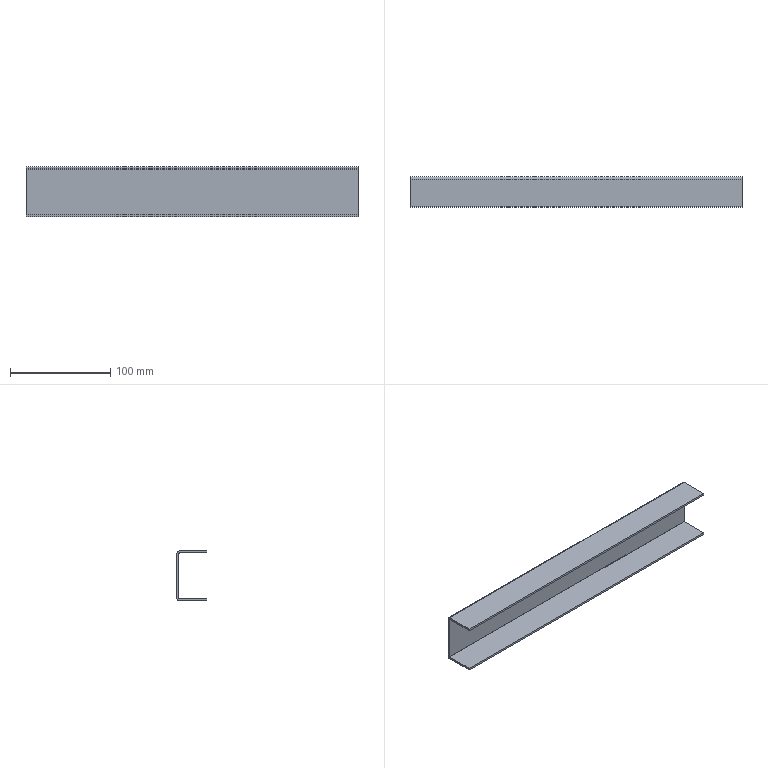Part | SolidWorks | 1 solid | 22 faces | box 332 x 30 x 50 mm | volume 69757 mm3 | plane 18 | cylinder 4 | commonest cylinder face diameters 0.2 x2 4.2 x2
STEP:
#1=CARTESIAN_POINT('',(166.,0.,-2.1));
#2=VERTEX_POINT('',#1);
#3=CARTESIAN_POINT('',(166.,-2.,-2.1));
#4=VERTEX_POINT('',#3);
#5=CARTESIAN_POINT('',(166.,0.,-2.1));
#6=DIRECTION('',(0.,-1.,0.));
#7=VECTOR('',#6,1000.);
#8=LINE('',#5,#7);
#9=EDGE_CURVE('',#2,#4,#8,.T.);
#10=ORIENTED_EDGE('',*,*,#9,.F.);
#11=CARTESIAN_POINT('',(166.,-2.1,0.));
#12=VERTEX_POINT('',#11);
#13=CARTESIAN_POINT('',(166.,-2.1,-2.1));
#14=DIRECTION('',(1.,0.,0.));
#15=DIRECTION('',(0.,0.,-1.));
#16=AXIS2_PLACEMENT_3D('',#13,#14,#15);
#17=CIRCLE('',#16,2.1);
#18=EDGE_CURVE('',#2,#12,#17,.T.);
#19=ORIENTED_EDGE('',*,*,#18,.T.);
#20=CARTESIAN_POINT('',(166.,-2.1,-2.));
#21=VERTEX_POINT('',#20);
#22=CARTESIAN_POINT('',(166.,-2.1,-2.));
#23=DIRECTION('',(0.,0.,1.));
#24=VECTOR('',#23,1000.);
#25=LINE('',#22,#24);
#26=EDGE_CURVE('',#21,#12,#25,.T.);
#27=ORIENTED_EDGE('',*,*,#26,.F.);
#28=CARTESIAN_POINT('',(166.,-2.1,-2.1));
#29=DIRECTION('',(1.,0.,0.));
#30=DIRECTION('',(0.,0.,-1.));
#31=AXIS2_PLACEMENT_3D('',#28,#29,#30);
#32=CIRCLE('',#31,0.1);
#33=EDGE_CURVE('',#4,#21,#32,.T.);
#34=ORIENTED_EDGE('',*,*,#33,.F.);
#35=EDGE_LOOP('',(#10,#19,#27,#34));
#36=FACE_OUTER_BOUND('',#35,.T.);
#37=CARTESIAN_POINT('',(166.,0.,-2.1));
#38=DIRECTION('',(1.,0.,0.));
#39=DIRECTION('',(0.,0.,-1.));
#40=AXIS2_PLACEMENT_3D('',#37,#38,#39);
#41=PLANE('',#40);
#42=ADVANCED_FACE('',(#36),#41,.T.);
#43=CARTESIAN_POINT('',(166.,0.,-47.9));
#44=VERTEX_POINT('',#43);
#45=CARTESIAN_POINT('',(166.,0.,0.));
#46=DIRECTION('',(0.,0.,1.));
#47=VECTOR('',#46,1000.);
#48=LINE('',#45,#47);
#49=EDGE_CURVE('',#44,#2,#48,.T.);
#50=ORIENTED_EDGE('',*,*,#49,.T.);
#51=ORIENTED_EDGE('',*,*,#9,.T.);
#52=CARTESIAN_POINT('',(166.,-2.,-47.9));
#53=VERTEX_POINT('',#52);
#54=CARTESIAN_POINT('',(166.,-2.,0.));
#55=DIRECTION('',(0.,0.,1.));
#56=VECTOR('',#55,1000.);
#57=LINE('',#54,#56);
#58=EDGE_CURVE('',#53,#4,#57,.T.);
#59=ORIENTED_EDGE('',*,*,#58,.F.);
#60=CARTESIAN_POINT('',(166.,-2.,-47.9));
#61=DIRECTION('',(0.,1.,0.));
#62=VECTOR('',#61,1000.);
#63=LINE('',#60,#62);
#64=EDGE_CURVE('',#53,#44,#63,.T.);
#65=ORIENTED_EDGE('',*,*,#64,.T.);
#66=EDGE_LOOP('',(#50,#51,#59,#65));
#67=FACE_OUTER_BOUND('',#66,.T.);
#68=CARTESIAN_POINT('',(166.,-2.1,-2.));
#69=DIRECTION('',(1.,0.,0.));
#70=DIRECTION('',(0.,0.,-1.));
#71=AXIS2_PLACEMENT_3D('',#68,#69,#70);
#72=PLANE('',#71);
#73=ADVANCED_FACE('',(#67),#72,.T.);
#74=CARTESIAN_POINT('',(-166.,-2.1,0.));
#75=VERTEX_POINT('',#74);
#76=CARTESIAN_POINT('',(-166.,-2.1,-2.));
#77=VERTEX_POINT('',#76);
#78=CARTESIAN_POINT('',(-166.,-2.1,0.));
#79=DIRECTION('',(0.,0.,-1.));
#80=VECTOR('',#79,1000.);
#81=LINE('',#78,#80);
#82=EDGE_CURVE('',#75,#77,#81,.T.);
#83=ORIENTED_EDGE('',*,*,#82,.F.);
#84=CARTESIAN_POINT('',(-166.,0.,-2.1));
#85=VERTEX_POINT('',#84);
#86=CARTESIAN_POINT('',(-166.,-2.1,-2.1));
#87=DIRECTION('',(1.,0.,0.));
#88=DIRECTION('',(0.,0.,-1.));
#89=AXIS2_PLACEMENT_3D('',#86,#87,#88);
#90=CIRCLE('',#89,2.1);
#91=EDGE_CURVE('',#85,#75,#90,.T.);
#92=ORIENTED_EDGE('',*,*,#91,.F.);
#93=CARTESIAN_POINT('',(-166.,-2.,-2.1));
#94=VERTEX_POINT('',#93);
#95=CARTESIAN_POINT('',(-166.,-2.,-2.1));
#96=DIRECTION('',(0.,1.,0.));
#97=VECTOR('',#96,1000.);
#98=LINE('',#95,#97);
#99=EDGE_CURVE('',#94,#85,#98,.T.);
#100=ORIENTED_EDGE('',*,*,#99,.F.);
#101=CARTESIAN_POINT('',(-166.,-2.1,-2.1));
#102=DIRECTION('',(1.,0.,0.));
#103=DIRECTION('',(0.,0.,-1.));
#104=AXIS2_PLACEMENT_3D('',#101,#102,#103);
#105=CIRCLE('',#104,0.1);
#106=EDGE_CURVE('',#94,#77,#105,.T.);
#107=ORIENTED_EDGE('',*,*,#106,.T.);
#108=EDGE_LOOP('',(#83,#92,#100,#107));
#109=FACE_OUTER_BOUND('',#108,.T.);
#110=CARTESIAN_POINT('',(-166.,-2.1,0.));
#111=DIRECTION('',(-1.,0.,0.));
#112=DIRECTION('',(0.,0.,1.));
#113=AXIS2_PLACEMENT_3D('',#110,#111,#112);
#114=PLANE('',#113);
#115=ADVANCED_FACE('',(#109),#114,.T.);
#116=CARTESIAN_POINT('',(-166.,-30.,0.));
#117=VERTEX_POINT('',#116);
#118=CARTESIAN_POINT('',(-166.,0.,0.));
#119=DIRECTION('',(0.,-1.,0.));
#120=VECTOR('',#119,1000.);
#121=LINE('',#118,#120);
#122=EDGE_CURVE('',#75,#117,#121,.T.);
#123=ORIENTED_EDGE('',*,*,#122,.F.);
#124=ORIENTED_EDGE('',*,*,#82,.T.);
#125=CARTESIAN_POINT('',(-166.,-30.,-2.));
#126=VERTEX_POINT('',#125);
#127=CARTESIAN_POINT('',(-166.,0.,-2.));
#128=DIRECTION('',(0.,-1.,0.));
#129=VECTOR('',#128,1000.);
#130=LINE('',#127,#129);
#131=EDGE_CURVE('',#77,#126,#130,.T.);
#132=ORIENTED_EDGE('',*,*,#131,.T.);
#133=CARTESIAN_POINT('',(-166.,-30.,-2.));
#134=DIRECTION('',(0.,0.,1.));
#135=VECTOR('',#134,1000.);
#136=LINE('',#133,#135);
#137=EDGE_CURVE('',#126,#117,#136,.T.);
#138=ORIENTED_EDGE('',*,*,#137,.T.);
#139=EDGE_LOOP('',(#123,#124,#132,#138));
#140=FACE_OUTER_BOUND('',#139,.T.);
#141=CARTESIAN_POINT('',(-166.,-2.,-2.1));
#142=DIRECTION('',(-1.,0.,0.));
#143=DIRECTION('',(0.,0.,1.));
#144=AXIS2_PLACEMENT_3D('',#141,#142,#143);
#145=PLANE('',#144);
#146=ADVANCED_FACE('',(#140),#145,.T.);
#147=CARTESIAN_POINT('',(166.,-2.1,-50.));
#148=VERTEX_POINT('',#147);
#149=CARTESIAN_POINT('',(166.,-2.1,-48.));
#150=VERTEX_POINT('',#149);
#151=CARTESIAN_POINT('',(166.,-2.1,-50.));
#152=DIRECTION('',(0.,0.,1.));
#153=VECTOR('',#152,1000.);
#154=LINE('',#151,#153);
#155=EDGE_CURVE('',#148,#150,#154,.T.);
#156=ORIENTED_EDGE('',*,*,#155,.F.);
#157=CARTESIAN_POINT('',(166.,-2.1,-47.9));
#158=DIRECTION('',(1.,0.,0.));
#159=DIRECTION('',(0.,0.,-1.));
#160=AXIS2_PLACEMENT_3D('',#157,#158,#159);
#161=CIRCLE('',#160,2.1);
#162=EDGE_CURVE('',#148,#44,#161,.T.);
#163=ORIENTED_EDGE('',*,*,#162,.T.);
#164=ORIENTED_EDGE('',*,*,#64,.F.);
#165=CARTESIAN_POINT('',(166.,-2.1,-47.9));
#166=DIRECTION('',(1.,0.,0.));
#167=DIRECTION('',(0.,0.,-1.));
#168=AXIS2_PLACEMENT_3D('',#165,#166,#167);
#169=CIRCLE('',#168,0.1);
#170=EDGE_CURVE('',#150,#53,#169,.T.);
#171=ORIENTED_EDGE('',*,*,#170,.F.);
#172=EDGE_LOOP('',(#156,#163,#164,#171));
#173=FACE_OUTER_BOUND('',#172,.T.);
#174=CARTESIAN_POINT('',(166.,-2.1,-50.));
#175=DIRECTION('',(1.,0.,0.));
#176=DIRECTION('',(0.,0.,-1.));
#177=AXIS2_PLACEMENT_3D('',#174,#175,#176);
#178=PLANE('',#177);
#179=ADVANCED_FACE('',(#173),#178,.T.);
#180=CARTESIAN_POINT('',(166.,-30.,-50.));
#181=VERTEX_POINT('',#180);
#182=CARTESIAN_POINT('',(166.,0.,-50.));
#183=DIRECTION('',(0.,1.,0.));
#184=VECTOR('',#183,1000.);
#185=LINE('',#182,#184);
#186=EDGE_CURVE('',#181,#148,#185,.T.);
#187=ORIENTED_EDGE('',*,*,#186,.T.);
#188=ORIENTED_EDGE('',*,*,#155,.T.);
#189=CARTESIAN_POINT('',(166.,-30.,-48.));
#190=VERTEX_POINT('',#189);
#191=CARTESIAN_POINT('',(166.,0.,-48.));
#192=DIRECTION('',(0.,1.,0.));
#193=VECTOR('',#192,1000.);
#194=LINE('',#191,#193);
#195=EDGE_CURVE('',#190,#150,#194,.T.);
#196=ORIENTED_EDGE('',*,*,#195,.F.);
#197=CARTESIAN_POINT('',(166.,-30.,-50.));
#198=DIRECTION('',(0.,0.,1.));
#199=VECTOR('',#198,1000.);
#200=LINE('',#197,#199);
#201=EDGE_CURVE('',#181,#190,#200,.T.);
#202=ORIENTED_EDGE('',*,*,#201,.F.);
#203=EDGE_LOOP('',(#187,#188,#196,#202));
#204=FACE_OUTER_BOUND('',#203,.T.);
#205=CARTESIAN_POINT('',(166.,-2.,-47.9));
#206=DIRECTION('',(1.,0.,0.));
#207=DIRECTION('',(0.,0.,-1.));
#208=AXIS2_PLACEMENT_3D('',#205,#206,#207);
#209=PLANE('',#208);
#210=ADVANCED_FACE('',(#204),#209,.T.);
#211=CARTESIAN_POINT('',(-166.,0.,-47.9));
#212=VERTEX_POINT('',#211);
#213=CARTESIAN_POINT('',(-166.,-2.,-47.9));
#214=VERTEX_POINT('',#213);
#215=CARTESIAN_POINT('',(-166.,0.,-47.9));
#216=DIRECTION('',(0.,-1.,0.));
#217=VECTOR('',#216,1000.);
#218=LINE('',#215,#217);
#219=EDGE_CURVE('',#212,#214,#218,.T.);
#220=ORIENTED_EDGE('',*,*,#219,.F.);
#221=CARTESIAN_POINT('',(-166.,-2.1,-50.));
#222=VERTEX_POINT('',#221);
#223=CARTESIAN_POINT('',(-166.,-2.1,-47.9));
#224=DIRECTION('',(1.,0.,0.));
#225=DIRECTION('',(0.,0.,-1.));
#226=AXIS2_PLACEMENT_3D('',#223,#224,#225);
#227=CIRCLE('',#226,2.1);
#228=EDGE_CURVE('',#222,#212,#227,.T.);
#229=ORIENTED_EDGE('',*,*,#228,.F.);
#230=CARTESIAN_POINT('',(-166.,-2.1,-48.));
#231=VERTEX_POINT('',#230);
#232=CARTESIAN_POINT('',(-166.,-2.1,-48.));
#233=DIRECTION('',(0.,0.,-1.));
#234=VECTOR('',#233,1000.);
#235=LINE('',#232,#234);
#236=EDGE_CURVE('',#231,#222,#235,.T.);
#237=ORIENTED_EDGE('',*,*,#236,.F.);
#238=CARTESIAN_POINT('',(-166.,-2.1,-47.9));
#239=DIRECTION('',(1.,0.,0.));
#240=DIRECTION('',(0.,0.,-1.));
#241=AXIS2_PLACEMENT_3D('',#238,#239,#240);
#242=CIRCLE('',#241,0.1);
#243=EDGE_CURVE('',#231,#214,#242,.T.);
#244=ORIENTED_EDGE('',*,*,#243,.T.);
#245=EDGE_LOOP('',(#220,#229,#237,#244));
#246=FACE_OUTER_BOUND('',#245,.T.);
#247=CARTESIAN_POINT('',(-166.,0.,-47.9));
#248=DIRECTION('',(-1.,0.,0.));
#249=DIRECTION('',(0.,0.,1.));
#250=AXIS2_PLACEMENT_3D('',#247,#248,#249);
#251=PLANE('',#250);
#252=ADVANCED_FACE('',(#246),#251,.T.);
#253=CARTESIAN_POINT('',(-166.,0.,0.));
#254=DIRECTION('',(0.,0.,1.));
#255=VECTOR('',#254,1000.);
#256=LINE('',#253,#255);
#257=EDGE_CURVE('',#212,#85,#256,.T.);
#258=ORIENTED_EDGE('',*,*,#257,.F.);
#259=ORIENTED_EDGE('',*,*,#219,.T.);
#260=CARTESIAN_POINT('',(-166.,-2.,0.));
#261=DIRECTION('',(0.,0.,1.));
#262=VECTOR('',#261,1000.);
#263=LINE('',#260,#262);
#264=EDGE_CURVE('',#214,#94,#263,.T.);
#265=ORIENTED_EDGE('',*,*,#264,.T.);
#266=ORIENTED_EDGE('',*,*,#99,.T.);
#267=EDGE_LOOP('',(#258,#259,#265,#266));
#268=FACE_OUTER_BOUND('',#267,.T.);
#269=CARTESIAN_POINT('',(-166.,-2.1,-48.));
#270=DIRECTION('',(-1.,0.,0.));
#271=DIRECTION('',(0.,0.,1.));
#272=AXIS2_PLACEMENT_3D('',#269,#270,#271);
#273=PLANE('',#272);
#274=ADVANCED_FACE('',(#268),#273,.T.);
#275=ORIENTED_EDGE('',*,*,#122,.T.);
#276=CARTESIAN_POINT('',(166.,-30.,0.));
#277=VERTEX_POINT('',#276);
#278=CARTESIAN_POINT('',(166.,-30.,0.));
#279=DIRECTION('',(-1.,0.,0.));
#280=VECTOR('',#279,1000.);
#281=LINE('',#278,#280);
#282=EDGE_CURVE('',#277,#117,#281,.T.);
#283=ORIENTED_EDGE('',*,*,#282,.F.);
#284=CARTESIAN_POINT('',(166.,0.,0.));
#285=DIRECTION('',(0.,-1.,0.));
#286=VECTOR('',#285,1000.);
#287=LINE('',#284,#286);
#288=EDGE_CURVE('',#12,#277,#287,.T.);
#289=ORIENTED_EDGE('',*,*,#288,.F.);
#290=CARTESIAN_POINT('',(166.,-2.1,0.));
#291=DIRECTION('',(-1.,0.,0.));
#292=VECTOR('',#291,1000.);
#293=LINE('',#290,#292);
#294=EDGE_CURVE('',#12,#75,#293,.T.);
#295=ORIENTED_EDGE('',*,*,#294,.T.);
#296=EDGE_LOOP('',(#275,#283,#289,#295));
#297=FACE_OUTER_BOUND('',#296,.T.);
#298=CARTESIAN_POINT('',(166.,0.,0.));
#299=DIRECTION('',(0.,0.,-1.));
#300=DIRECTION('',(0.,1.,0.));
#301=AXIS2_PLACEMENT_3D('',#298,#299,#300);
#302=PLANE('',#301);
#303=ADVANCED_FACE('',(#297),#302,.F.);
#304=ORIENTED_EDGE('',*,*,#137,.F.);
#305=CARTESIAN_POINT('',(166.,-30.,-2.));
#306=VERTEX_POINT('',#305);
#307=CARTESIAN_POINT('',(166.,-30.,-2.));
#308=DIRECTION('',(-1.,0.,0.));
#309=VECTOR('',#308,1000.);
#310=LINE('',#307,#309);
#311=EDGE_CURVE('',#306,#126,#310,.T.);
#312=ORIENTED_EDGE('',*,*,#311,.F.);
#313=CARTESIAN_POINT('',(166.,-30.,-2.));
#314=DIRECTION('',(0.,0.,1.));
#315=VECTOR('',#314,1000.);
#316=LINE('',#313,#315);
#317=EDGE_CURVE('',#306,#277,#316,.T.);
#318=ORIENTED_EDGE('',*,*,#317,.T.);
#319=ORIENTED_EDGE('',*,*,#282,.T.);
#320=EDGE_LOOP('',(#304,#312,#318,#319));
#321=FACE_OUTER_BOUND('',#320,.T.);
#322=CARTESIAN_POINT('',(166.,-30.,-2.));
#323=DIRECTION('',(0.,-1.,0.));
#324=DIRECTION('',(0.,0.,-1.));
#325=AXIS2_PLACEMENT_3D('',#322,#323,#324);
#326=PLANE('',#325);
#327=ADVANCED_FACE('',(#321),#326,.T.);
#328=ORIENTED_EDGE('',*,*,#131,.F.);
#329=CARTESIAN_POINT('',(166.,-2.1,-2.));
#330=DIRECTION('',(-1.,0.,0.));
#331=VECTOR('',#330,1000.);
#332=LINE('',#329,#331);
#333=EDGE_CURVE('',#21,#77,#332,.T.);
#334=ORIENTED_EDGE('',*,*,#333,.F.);
#335=CARTESIAN_POINT('',(166.,0.,-2.));
#336=DIRECTION('',(0.,-1.,0.));
#337=VECTOR('',#336,1000.);
#338=LINE('',#335,#337);
#339=EDGE_CURVE('',#21,#306,#338,.T.);
#340=ORIENTED_EDGE('',*,*,#339,.T.);
#341=ORIENTED_EDGE('',*,*,#311,.T.);
#342=EDGE_LOOP('',(#328,#334,#340,#341));
#343=FACE_OUTER_BOUND('',#342,.T.);
#344=CARTESIAN_POINT('',(166.,0.,-2.));
#345=DIRECTION('',(0.,0.,-1.));
#346=DIRECTION('',(0.,1.,0.));
#347=AXIS2_PLACEMENT_3D('',#344,#345,#346);
#348=PLANE('',#347);
#349=ADVANCED_FACE('',(#343),#348,.T.);
#350=ORIENTED_EDGE('',*,*,#106,.F.);
#351=CARTESIAN_POINT('',(166.,-2.,-2.1));
#352=DIRECTION('',(-1.,0.,0.));
#353=VECTOR('',#352,1000.);
#354=LINE('',#351,#353);
#355=EDGE_CURVE('',#4,#94,#354,.T.);
#356=ORIENTED_EDGE('',*,*,#355,.F.);
#357=ORIENTED_EDGE('',*,*,#33,.T.);
#358=ORIENTED_EDGE('',*,*,#333,.T.);
#359=EDGE_LOOP('',(#350,#356,#357,#358));
#360=FACE_OUTER_BOUND('',#359,.T.);
#361=CARTESIAN_POINT('',(166.,-2.1,-2.1));
#362=DIRECTION('',(-1.,0.,0.));
#363=DIRECTION('',(0.,0.,1.));
#364=AXIS2_PLACEMENT_3D('',#361,#362,#363);
#365=CYLINDRICAL_SURFACE('',#364,0.1);
#366=ADVANCED_FACE('',(#360),#365,.F.);
#367=ORIENTED_EDGE('',*,*,#264,.F.);
#368=CARTESIAN_POINT('',(166.,-2.,-47.9));
#369=DIRECTION('',(-1.,0.,0.));
#370=VECTOR('',#369,1000.);
#371=LINE('',#368,#370);
#372=EDGE_CURVE('',#53,#214,#371,.T.);
#373=ORIENTED_EDGE('',*,*,#372,.F.);
#374=ORIENTED_EDGE('',*,*,#58,.T.);
#375=ORIENTED_EDGE('',*,*,#355,.T.);
#376=EDGE_LOOP('',(#367,#373,#374,#375));
#377=FACE_OUTER_BOUND('',#376,.T.);
#378=CARTESIAN_POINT('',(166.,-2.,0.));
#379=DIRECTION('',(0.,-1.,0.));
#380=DIRECTION('',(0.,0.,-1.));
#381=AXIS2_PLACEMENT_3D('',#378,#379,#380);
#382=PLANE('',#381);
#383=ADVANCED_FACE('',(#377),#382,.T.);
#384=ORIENTED_EDGE('',*,*,#243,.F.);
#385=CARTESIAN_POINT('',(166.,-2.1,-48.));
#386=DIRECTION('',(-1.,0.,0.));
#387=VECTOR('',#386,1000.);
#388=LINE('',#385,#387);
#389=EDGE_CURVE('',#150,#231,#388,.T.);
#390=ORIENTED_EDGE('',*,*,#389,.F.);
#391=ORIENTED_EDGE('',*,*,#170,.T.);
#392=ORIENTED_EDGE('',*,*,#372,.T.);
#393=EDGE_LOOP('',(#384,#390,#391,#392));
#394=FACE_OUTER_BOUND('',#393,.T.);
#395=CARTESIAN_POINT('',(166.,-2.1,-47.9));
#396=DIRECTION('',(-1.,0.,0.));
#397=DIRECTION('',(0.,0.,1.));
#398=AXIS2_PLACEMENT_3D('',#395,#396,#397);
#399=CYLINDRICAL_SURFACE('',#398,0.1);
#400=ADVANCED_FACE('',(#394),#399,.F.);
#401=CARTESIAN_POINT('',(-166.,-30.,-48.));
#402=VERTEX_POINT('',#401);
#403=CARTESIAN_POINT('',(-166.,0.,-48.));
#404=DIRECTION('',(0.,1.,0.));
#405=VECTOR('',#404,1000.);
#406=LINE('',#403,#405);
#407=EDGE_CURVE('',#402,#231,#406,.T.);
#408=ORIENTED_EDGE('',*,*,#407,.F.);
#409=CARTESIAN_POINT('',(166.,-30.,-48.));
#410=DIRECTION('',(-1.,0.,0.));
#411=VECTOR('',#410,1000.);
#412=LINE('',#409,#411);
#413=EDGE_CURVE('',#190,#402,#412,.T.);
#414=ORIENTED_EDGE('',*,*,#413,.F.);
#415=ORIENTED_EDGE('',*,*,#195,.T.);
#416=ORIENTED_EDGE('',*,*,#389,.T.);
#417=EDGE_LOOP('',(#408,#414,#415,#416));
#418=FACE_OUTER_BOUND('',#417,.T.);
#419=CARTESIAN_POINT('',(166.,0.,-48.));
#420=DIRECTION('',(0.,0.,1.));
#421=DIRECTION('',(0.,-1.,0.));
#422=AXIS2_PLACEMENT_3D('',#419,#420,#421);
#423=PLANE('',#422);
#424=ADVANCED_FACE('',(#418),#423,.T.);
#425=CARTESIAN_POINT('',(-166.,-30.,-50.));
#426=VERTEX_POINT('',#425);
#427=CARTESIAN_POINT('',(-166.,-30.,-50.));
#428=DIRECTION('',(0.,0.,1.));
#429=VECTOR('',#428,1000.);
#430=LINE('',#427,#429);
#431=EDGE_CURVE('',#426,#402,#430,.T.);
#432=ORIENTED_EDGE('',*,*,#431,.F.);
#433=CARTESIAN_POINT('',(166.,-30.,-50.));
#434=DIRECTION('',(-1.,0.,0.));
#435=VECTOR('',#434,1000.);
#436=LINE('',#433,#435);
#437=EDGE_CURVE('',#181,#426,#436,.T.);
#438=ORIENTED_EDGE('',*,*,#437,.F.);
#439=ORIENTED_EDGE('',*,*,#201,.T.);
#440=ORIENTED_EDGE('',*,*,#413,.T.);
#441=EDGE_LOOP('',(#432,#438,#439,#440));
#442=FACE_OUTER_BOUND('',#441,.T.);
#443=CARTESIAN_POINT('',(166.,-30.,-50.));
#444=DIRECTION('',(0.,-1.,0.));
#445=DIRECTION('',(0.,0.,-1.));
#446=AXIS2_PLACEMENT_3D('',#443,#444,#445);
#447=PLANE('',#446);
#448=ADVANCED_FACE('',(#442),#447,.T.);
#449=CARTESIAN_POINT('',(-166.,0.,-50.));
#450=DIRECTION('',(0.,1.,0.));
#451=VECTOR('',#450,1000.);
#452=LINE('',#449,#451);
#453=EDGE_CURVE('',#426,#222,#452,.T.);
#454=ORIENTED_EDGE('',*,*,#453,.T.);
#455=CARTESIAN_POINT('',(166.,-2.1,-50.));
#456=DIRECTION('',(-1.,0.,0.));
#457=VECTOR('',#456,1000.);
#458=LINE('',#455,#457);
#459=EDGE_CURVE('',#148,#222,#458,.T.);
#460=ORIENTED_EDGE('',*,*,#459,.F.);
#461=ORIENTED_EDGE('',*,*,#186,.F.);
#462=ORIENTED_EDGE('',*,*,#437,.T.);
#463=EDGE_LOOP('',(#454,#460,#461,#462));
#464=FACE_OUTER_BOUND('',#463,.T.);
#465=CARTESIAN_POINT('',(166.,0.,-50.));
#466=DIRECTION('',(0.,0.,1.));
#467=DIRECTION('',(0.,-1.,0.));
#468=AXIS2_PLACEMENT_3D('',#465,#466,#467);
#469=PLANE('',#468);
#470=ADVANCED_FACE('',(#464),#469,.F.);
#471=ORIENTED_EDGE('',*,*,#228,.T.);
#472=CARTESIAN_POINT('',(166.,0.,-47.9));
#473=DIRECTION('',(-1.,0.,0.));
#474=VECTOR('',#473,1000.);
#475=LINE('',#472,#474);
#476=EDGE_CURVE('',#44,#212,#475,.T.);
#477=ORIENTED_EDGE('',*,*,#476,.F.);
#478=ORIENTED_EDGE('',*,*,#162,.F.);
#479=ORIENTED_EDGE('',*,*,#459,.T.);
#480=EDGE_LOOP('',(#471,#477,#478,#479));
#481=FACE_OUTER_BOUND('',#480,.T.);
#482=CARTESIAN_POINT('',(166.,-2.1,-47.9));
#483=DIRECTION('',(-1.,0.,0.));
#484=DIRECTION('',(0.,0.,1.));
#485=AXIS2_PLACEMENT_3D('',#482,#483,#484);
#486=CYLINDRICAL_SURFACE('',#485,2.1);
#487=ADVANCED_FACE('',(#481),#486,.T.);
#488=ORIENTED_EDGE('',*,*,#257,.T.);
#489=CARTESIAN_POINT('',(166.,0.,-2.1));
#490=DIRECTION('',(-1.,0.,0.));
#491=VECTOR('',#490,1000.);
#492=LINE('',#489,#491);
#493=EDGE_CURVE('',#2,#85,#492,.T.);
#494=ORIENTED_EDGE('',*,*,#493,.F.);
#495=ORIENTED_EDGE('',*,*,#49,.F.);
#496=ORIENTED_EDGE('',*,*,#476,.T.);
#497=EDGE_LOOP('',(#488,#494,#495,#496));
#498=FACE_OUTER_BOUND('',#497,.T.);
#499=CARTESIAN_POINT('',(166.,0.,0.));
#500=DIRECTION('',(0.,-1.,0.));
#501=DIRECTION('',(0.,0.,-1.));
#502=AXIS2_PLACEMENT_3D('',#499,#500,#501);
#503=PLANE('',#502);
#504=ADVANCED_FACE('',(#498),#503,.F.);
#505=ORIENTED_EDGE('',*,*,#91,.T.);
#506=ORIENTED_EDGE('',*,*,#294,.F.);
#507=ORIENTED_EDGE('',*,*,#18,.F.);
#508=ORIENTED_EDGE('',*,*,#493,.T.);
#509=EDGE_LOOP('',(#505,#506,#507,#508));
#510=FACE_OUTER_BOUND('',#509,.T.);
#511=CARTESIAN_POINT('',(166.,-2.1,-2.1));
#512=DIRECTION('',(-1.,0.,0.));
#513=DIRECTION('',(0.,0.,1.));
#514=AXIS2_PLACEMENT_3D('',#511,#512,#513);
#515=CYLINDRICAL_SURFACE('',#514,2.1);
#516=ADVANCED_FACE('',(#510),#515,.T.);
#517=ORIENTED_EDGE('',*,*,#288,.T.);
#518=ORIENTED_EDGE('',*,*,#317,.F.);
#519=ORIENTED_EDGE('',*,*,#339,.F.);
#520=ORIENTED_EDGE('',*,*,#26,.T.);
#521=EDGE_LOOP('',(#517,#518,#519,#520));
#522=FACE_OUTER_BOUND('',#521,.T.);
#523=CARTESIAN_POINT('',(166.,-2.1,-2.1));
#524=DIRECTION('',(1.,0.,0.));
#525=DIRECTION('',(0.,0.,-1.));
#526=AXIS2_PLACEMENT_3D('',#523,#524,#525);
#527=PLANE('',#526);
#528=ADVANCED_FACE('',(#522),#527,.T.);
#529=ORIENTED_EDGE('',*,*,#407,.T.);
#530=ORIENTED_EDGE('',*,*,#236,.T.);
#531=ORIENTED_EDGE('',*,*,#453,.F.);
#532=ORIENTED_EDGE('',*,*,#431,.T.);
#533=EDGE_LOOP('',(#529,#530,#531,#532));
#534=FACE_OUTER_BOUND('',#533,.T.);
#535=CARTESIAN_POINT('',(-166.,-2.1,-2.1));
#536=DIRECTION('',(1.,0.,0.));
#537=DIRECTION('',(0.,0.,-1.));
#538=AXIS2_PLACEMENT_3D('',#535,#536,#537);
#539=PLANE('',#538);
#540=ADVANCED_FACE('',(#534),#539,.F.);
#541=CLOSED_SHELL('',(#42,#73,#115,#146,#179,#210,#252,#274,#303,#327,#349,#366,#383,#400,#424,#448,#470,#487,#504,#516,#528,#540));
#542=MANIFOLD_SOLID_BREP('',#541);
#543=CARTESIAN_POINT('',(0.,0.,0.));
#544=DIRECTION('',(0.,0.,1.));
#545=DIRECTION('',(1.,0.,0.));
#546=AXIS2_PLACEMENT_3D('',#543,#544,#545);
#547=(LENGTH_UNIT()NAMED_UNIT(*)SI_UNIT(.MILLI.,.METRE.));
#548=UNCERTAINTY_MEASURE_WITH_UNIT(LENGTH_MEASURE(0.00001),#547,'','');
#549=(NAMED_UNIT(*)PLANE_ANGLE_UNIT()SI_UNIT($,.RADIAN.));
#550=(NAMED_UNIT(*)SI_UNIT($,.STERADIAN.)SOLID_ANGLE_UNIT());
#551=(GEOMETRIC_REPRESENTATION_CONTEXT(3)GLOBAL_UNCERTAINTY_ASSIGNED_CONTEXT((#548))GLOBAL_UNIT_ASSIGNED_CONTEXT((#547,#549,#550))REPRESENTATION_CONTEXT('',''));
#552=ADVANCED_BREP_SHAPE_REPRESENTATION('',(#542,#546),#551);